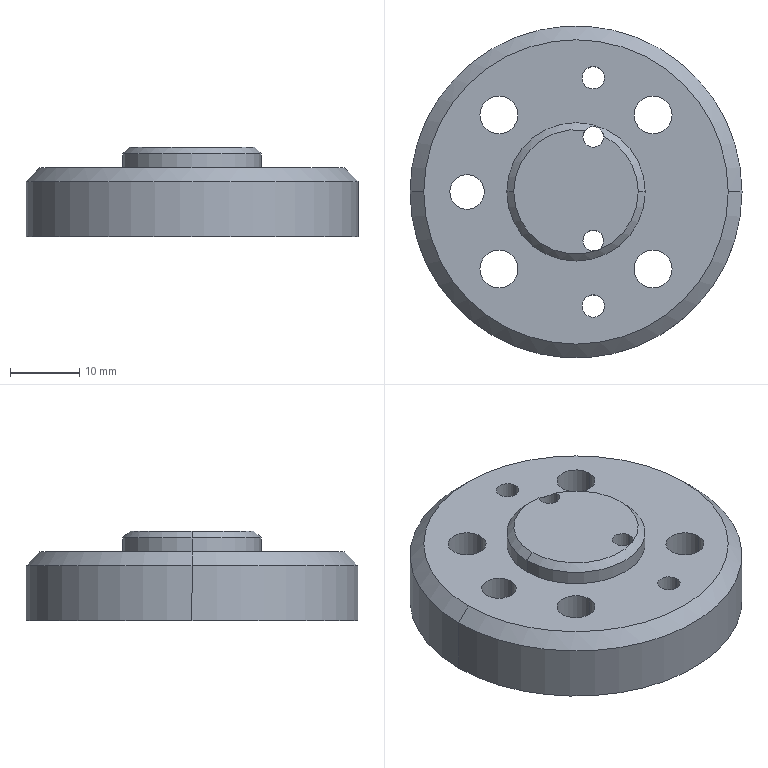Part | STEP file | ASND-0110-Body 1-22 | 1 solid | 41 faces | box 48 x 48 x 13 mm | volume 15905 mm3 | cylinder 30 | plane 7 | cone 4 | commonest cylinder face diameters 5.5 x8 10 x8 3 x4 3.242 x4 5 x2 20 x2